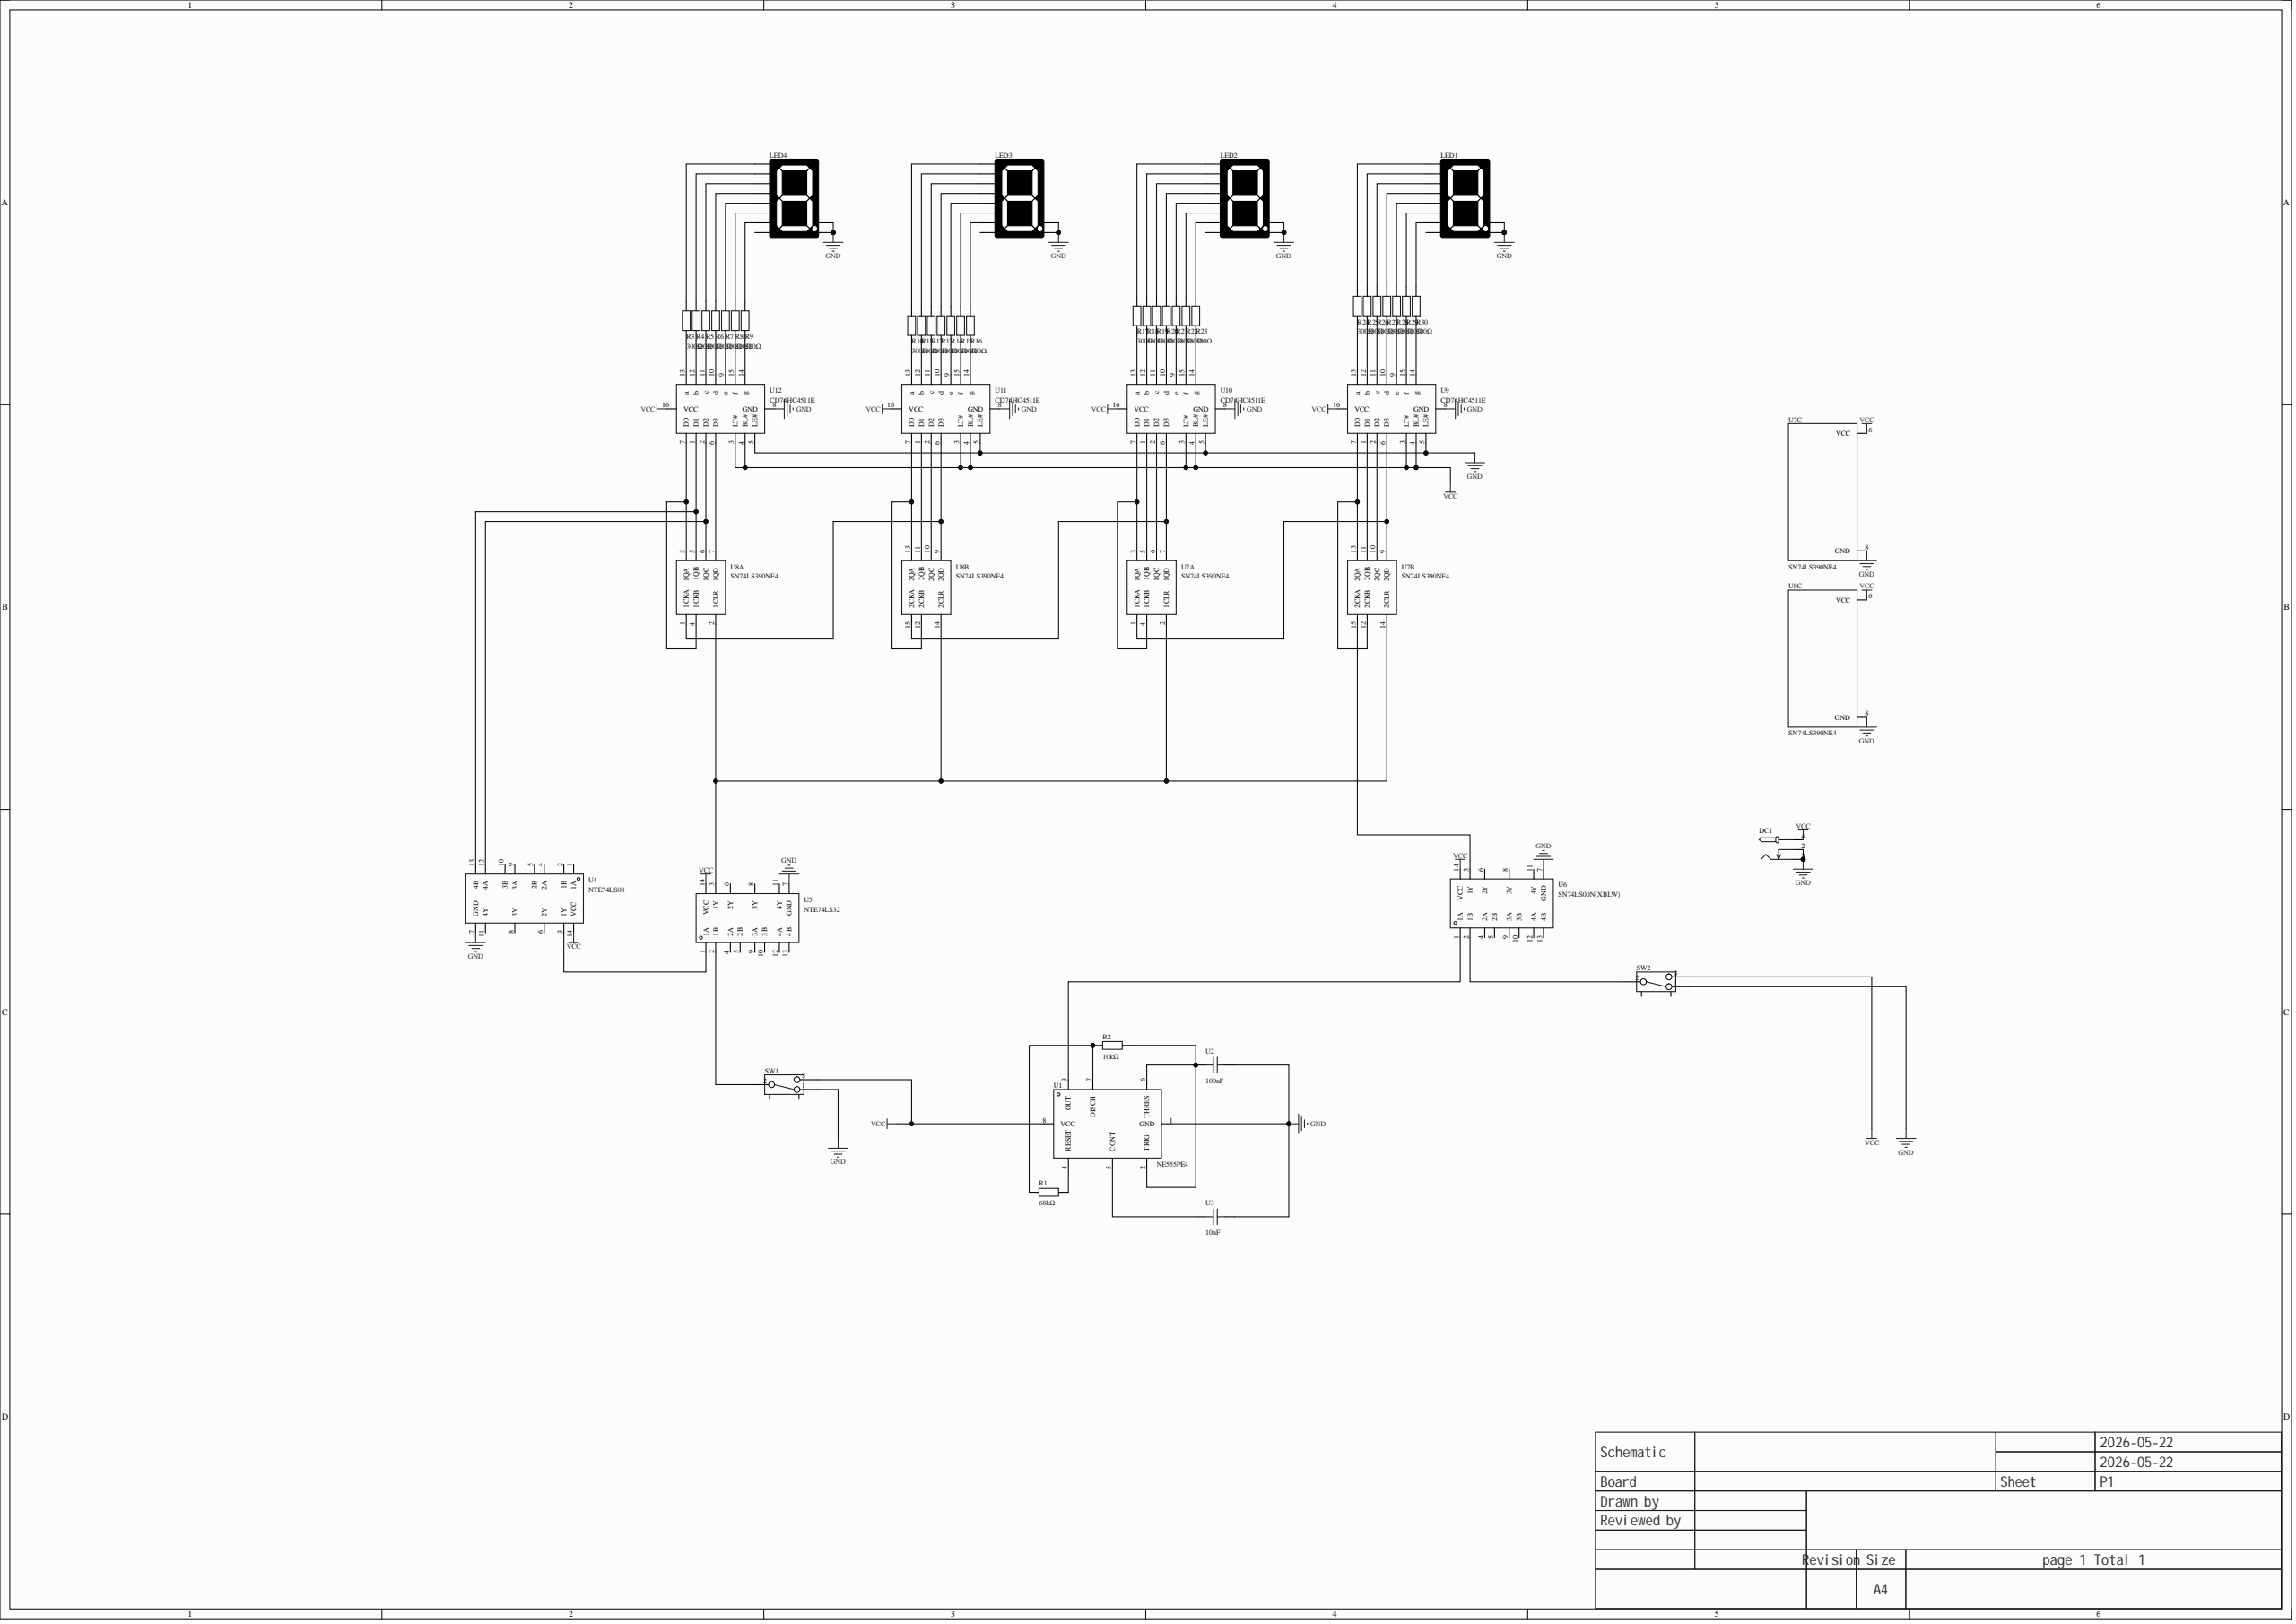Circuit board | Altium Designer | 49 parts | 84 nets
Bill of materials:
Comment,Description,Designator,Footprint,LibRef,Quantity
"","","DC1","DC-2.0","DC-005_2.0","1"
"","","LED1, LED2, LED3, LED4","LED-SEG-TH_10P-L12.6-W19.0-P2.54-S15.24-BL","LED_SEG_TH_0.56x1","4"
"68kΩ","","R1","Res_1/8W","Res_AXIAL-1/8W","1"
"10kΩ","","R2","Res_1/8W","Res_AXIAL-1/8W","1"
"300Ω","","R3, R4, R5, R6, R7, R8, R9, R10, R11, R12, R13, R14, R15, R16, R17, R18, R19, R20, R21, R22, R23, R24, R25, R26, R27, R28, R29, R30","Res_1/8W","Res_AXIAL-1/8W","28"
"","","SW1, SW2","拨动开关_侧","拨动开关_侧","2"
"NE555PE4","NE555 single timer","U1","PDIP-8_L9.6-W6.4-P2.54-LS7.9-BL-1","NE555PE4","1"
"100nF","","U2","CAP-TH_L5.0-W2.5-P5.00-D1.0","100nF","1"
"10nF","","U3","CAP-TH_L5.0-W2.5-P5.00-D1.0","100nF","1"
"NTE74LS08","Logic type: AND gate; channels: 4; operating voltage: 4.75V~5.25V; quiescent current (Iq): 8.8mA; propagation delay (tpd): 20ns@5V,15pF;","U4","DIP-14_L19.6-W6.4-P2.54-LS7.6-BL","NTE74LS08","1"
"NTE74LS32","Logic type: OR gate; channels: 4; operating voltage: 4.75V~5.25V; propagation delay (tpd): 22ns@5V,50pF;","U5","DIP-14_L19.6-W6.4-P2.54-LS7.6-BL","NTE74LS32","1"
"SN74LS00N(XBLW)","SN74LS00 is a quad 2-input NAND gate; inputs include clamp diodes, allowing current-limiting resistors to interface inputs to voltages above Vcc.","U6","PDIP-14_L19.3-W6.4-P2.54-LS7.6-BL","SN74LS00N(XBLW)","1"
"SN74LS390NE4","SN74LS390 dual 4-bit decade counter","U7, U8","PDIP-16_L19.3-W6.4-P2.54-LS7.94-BL","SN74LS390NE4","2"
"CD74HC4511E","CD74HC4511 high-speed CMOS logic BCD to 7-segment latch/decoder/driver","U9, U10, U11, U12","PDIP-16_L19.7-W6.6-P2.54-LS7.6-BL","CD74HC4511E","4"
Netlist (Protel format):
[
DC1
DC-2.0




]
[
LED1
LED-SEG-TH_10P-L12.6-W19.0-P2.54-S15.24-BL




]
[
LED2
LED-SEG-TH_10P-L12.6-W19.0-P2.54-S15.24-BL




]
[
LED3
LED-SEG-TH_10P-L12.6-W19.0-P2.54-S15.24-BL




]
[
LED4
LED-SEG-TH_10P-L12.6-W19.0-P2.54-S15.24-BL




]
[
R1
Res_1/8W
68kΩ



]
[
R2
Res_1/8W
10kΩ



]
[
R3
Res_1/8W
300Ω



]
[
R4
Res_1/8W
300Ω



]
[
R5
Res_1/8W
300Ω



]
[
R6
Res_1/8W
300Ω



]
[
R7
Res_1/8W
300Ω



]
[
R8
Res_1/8W
300Ω



]
[
R9
Res_1/8W
300Ω



]
[
R10
Res_1/8W
300Ω



]
[
R11
Res_1/8W
300Ω



]
[
R12
Res_1/8W
300Ω



]
[
R13
Res_1/8W
300Ω



]
[
R14
Res_1/8W
300Ω



]
[
R15
Res_1/8W
300Ω



]
[
R16
Res_1/8W
300Ω



]
[
R17
Res_1/8W
300Ω



]
[
R18
Res_1/8W
300Ω



]
[
R19
Res_1/8W
300Ω



]
[
R20
Res_1/8W
300Ω



]
[
R21
Res_1/8W
300Ω



]
[
R22
Res_1/8W
300Ω



]
[
R23
Res_1/8W
300Ω



]
[
R24
Res_1/8W
300Ω



]
[
R25
Res_1/8W
300Ω



]
[
R26
Res_1/8W
300Ω



]
[
R27
Res_1/8W
300Ω



]
[
R28
Res_1/8W
300Ω



]
[
R29
Res_1/8W
300Ω



]
[
R30
Res_1/8W
300Ω



]
[
SW1
拨动开关_侧




]
[
SW2
拨动开关_侧




]
[
U1
PDIP-8_L9.6-W6.4-P2.54-LS7.9-BL-1
NE555PE4



]
[
U2
CAP-TH_L5.0-W2.5-P5.00-D1.0
100nF



]
[
U3
CAP-TH_L5.0-W2.5-P5.00-D1.0
10nF



]
[
U4
DIP-14_L19.6-W6.4-P2.54-LS7.6-BL
NTE74LS08



]
[
U5
DIP-14_L19.6-W6.4-P2.54-LS7.6-BL
NTE74LS32



]
[
U6
PDIP-14_L19.3-W6.4-P2.54-LS7.6-BL
SN74LS00N(XBLW)



]
[
U7
PDIP-16_L19.3-W6.4-P2.54-LS7.94-BL
SN74LS390NE4



]
[
U8
PDIP-16_L19.3-W6.4-P2.54-LS7.94-BL
SN74LS390NE4



]
[
U9
PDIP-16_L19.7-W6.6-P2.54-LS7.6-BL
CD74HC4511E



]
[
U10
PDIP-16_L19.7-W6.6-P2.54-LS7.6-BL
CD74HC4511E



]
[
U11
PDIP-16_L19.7-W6.6-P2.54-LS7.6-BL
CD74HC4511E



]
[
U12
PDIP-16_L19.7-W6.6-P2.54-LS7.6-BL
CD74HC4511E



]
(
VCC
DC1-4
SW1-3
SW2-3
U1-8
U4-14
U5-14
U6-14
U7-16
U8-16
U9-3
U9-4
U9-16
U10-3
U10-4
U10-16
U11-3
U11-4
U11-16
U12-3
U12-4
U12-16
)
(
NetU8_12
U8-12
U8-13
U11-7
)
(
NetU8_11
U8-11
U11-1
)
(
NetU8_10
U8-10
U11-2
)
(
NetU8_7
U8-7
U12-6
)
(
NetU8_3
U8-3
U8-4
U12-7
)
(
NetU8_1
U8-1
U8-9
U11-6
)
(
NetU7_12
U7-12
U7-13
U9-7
)
(
NetU7_11
U7-11
U9-1
)
(
NetU7_10
U7-10
U9-2
)
(
NetU7_7
U7-7
U8-15
U10-6
)
(
NetU7_6
U7-6
U10-2
)
(
NetU7_5
U7-5
U10-1
)
(
NetU7_3
U7-3
U7-4
U10-7
)
(
NetU7_1
U7-1
U7-9
U9-6
)
(
NetU6_3
U6-3
U7-15
)
(
NetU5_3
U5-3
U7-2
U7-14
U8-2
U8-14
)
(
NetU4_13
U4-13
U8-5
U12-1
)
(
NetU4_12
U4-12
U8-6
U12-2
)
(
NetU4_3
U4-3
U5-1
)
(
NetU1_5
U1-5
U3-2
)
(
NetU1_3
U1-3
U6-1
)
(
NetSW2_2
SW2-2
U6-2
)
(
NetSW1_2
SW1-2
U5-2
)
(
NetR30_1
R30-1
U9-14
)
(
NetR29_1
R29-1
U9-15
)
(
NetR28_1
R28-1
U9-9
)
(
NetR27_1
R27-1
U9-10
)
(
NetR26_1
R26-1
U9-11
)
(
NetR25_1
R25-1
U9-12
)
(
NetR24_1
R24-1
U9-13
)
(
NetR23_1
R23-1
U10-14
)
(
NetR22_1
R22-1
U10-15
)
(
NetR21_1
R21-1
U10-9
)
(
NetR20_1
R20-1
U10-10
)
(
NetR19_1
R19-1
U10-11
)
(
NetR18_1
R18-1
U10-12
)
(
NetR17_1
R17-1
U10-13
)
(
NetR16_1
R16-1
U11-14
)
(
NetR15_1
R15-1
U11-15
)
(
NetR14_1
R14-1
U11-9
)
(
NetR13_1
R13-1
U11-10
)
(
NetR12_1
R12-1
U11-11
)
(
NetR11_1
R11-1
U11-12
)
(
NetR10_1
R10-1
U11-13
)
(
NetR9_1
R9-1
U12-14
)
(
NetR8_1
R8-1
U12-15
)
(
NetR7_1
R7-1
U12-9
)
(
NetR6_1
R6-1
U12-10
)
(
NetR5_1
R5-1
U12-11
)
(
NetR4_1
R4-1
U12-12
)
(
NetR3_1
R3-1
U12-13
)
(
NetR2_2
R2-2
U1-2
U1-6
U2-2
)
(
NetR1_2
R1-2
U1-4
)
(
NetR1_1
R1-1
R2-1
U1-7
)
(
NetLED4_10
LED4-10
R9-2
)
(
NetLED4_9
LED4-9
R8-2
)
(
NetLED4_7
LED4-7
R3-2
)
(
NetLED4_6
LED4-6
R4-2
)
(
NetLED4_4
LED4-4
R5-2
)
(
NetLED4_2
LED4-2
R6-2
)
(
NetLED4_1
LED4-1
R7-2
)
(
NetLED3_10
LED3-10
R16-2
)
(
NetLED3_9
LED3-9
R15-2
)
(
NetLED3_7
LED3-7
R10-2
)
(
NetLED3_6
LED3-6
R11-2
)
(
NetLED3_4
LED3-4
R12-2
)
(
NetLED3_2
LED3-2
R13-2
)
(
NetLED3_1
LED3-1
R14-2
)
(
NetLED2_10
LED2-10
R23-2
)
(
NetLED2_9
LED2-9
R22-2
)
(
NetLED2_7
LED2-7
R17-2
)
(
NetLED2_6
LED2-6
R18-2
)
(
NetLED2_4
LED2-4
R19-2
)
(
NetLED2_2
LED2-2
R20-2
)
(
NetLED2_1
LED2-1
R21-2
)
(
NetLED1_10
LED1-10
R30-2
)
(
NetLED1_9
LED1-9
R29-2
)
(
NetLED1_7
LED1-7
R24-2
)
(
NetLED1_6
LED1-6
R25-2
)
(
NetLED1_4
LED1-4
R26-2
)
(
NetLED1_2
LED1-2
R27-2
)
(
NetLED1_1
LED1-1
R28-2
)
(
GND
DC1-2
DC1-3
LED1-3
LED1-8
LED2-3
LED2-8
LED3-3
LED3-8
LED4-3
LED4-8
SW1-1
SW2-1
U1-1
U2-1
U3-1
U4-7
U5-7
U6-7
U7-8
U8-8
U9-5
U9-8
U10-5
U10-8
U11-5
U11-8
U12-5
U12-8
)